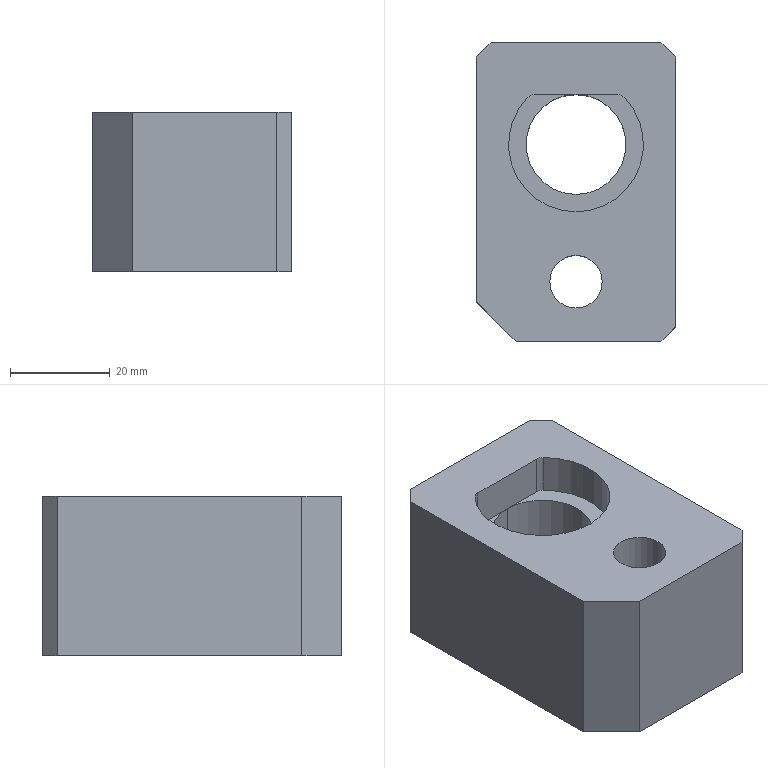Part | STEP file | lll_id3638_x_t | 1 solid | 21 faces | box 40 x 60 x 32 mm | volume 58416 mm3 | plane 13 | cylinder 8 | commonest cylinder face diameters 4 x2 20 x2 27 x2 10.5 x1 17 x1
STEP:
#1=CARTESIAN_POINT('',(3587.234,240.45,60.5));
#2=VERTEX_POINT('',#1);
#3=CARTESIAN_POINT('',(3587.234,220.45,60.5));
#4=VERTEX_POINT('',#3);
#5=CARTESIAN_POINT('',(3587.234,230.45,60.5));
#6=DIRECTION('',(0.,0.,-1.));
#7=DIRECTION('',(1.,0.,0.));
#8=AXIS2_PLACEMENT_3D('',#5,#6,#7);
#9=CIRCLE('',#8,10.);
#10=EDGE_CURVE('',#2,#4,#9,.T.);
#11=ORIENTED_EDGE('',*,*,#10,.F.);
#12=CARTESIAN_POINT('',(3587.234,230.45,60.5));
#13=DIRECTION('',(0.,0.,-1.));
#14=DIRECTION('',(1.,0.,0.));
#15=AXIS2_PLACEMENT_3D('',#12,#13,#14);
#16=CIRCLE('',#15,10.);
#17=EDGE_CURVE('',#4,#2,#16,.T.);
#18=ORIENTED_EDGE('',*,*,#17,.F.);
#19=EDGE_LOOP('',(#11,#18));
#20=FACE_BOUND('',#19,.T.);
#21=CARTESIAN_POINT('',(3567.234,198.95,60.5));
#22=VERTEX_POINT('',#21);
#23=CARTESIAN_POINT('',(3567.234,247.95,60.5));
#24=VERTEX_POINT('',#23);
#25=CARTESIAN_POINT('',(3567.234,199.225,60.5));
#26=DIRECTION('',(0.,1.,0.));
#27=VECTOR('',#26,1.);
#28=LINE('',#25,#27);
#29=EDGE_CURVE('',#22,#24,#28,.T.);
#30=ORIENTED_EDGE('',*,*,#29,.T.);
#31=CARTESIAN_POINT('',(3570.234,250.95,60.5));
#32=VERTEX_POINT('',#31);
#33=CARTESIAN_POINT('',(3570.234,250.95,60.5));
#34=DIRECTION('',(-0.7071,-0.7071,0.));
#35=VECTOR('',#34,1.);
#36=LINE('',#33,#35);
#37=EDGE_CURVE('',#32,#24,#36,.T.);
#38=ORIENTED_EDGE('',*,*,#37,.F.);
#39=CARTESIAN_POINT('',(3604.234,250.95,60.5));
#40=VERTEX_POINT('',#39);
#41=CARTESIAN_POINT('',(3587.234,250.95,60.5));
#42=DIRECTION('',(1.,0.,0.));
#43=VECTOR('',#42,1.);
#44=LINE('',#41,#43);
#45=EDGE_CURVE('',#32,#40,#44,.T.);
#46=ORIENTED_EDGE('',*,*,#45,.T.);
#47=CARTESIAN_POINT('',(3607.234,247.95,60.5));
#48=VERTEX_POINT('',#47);
#49=CARTESIAN_POINT('',(3607.234,247.95,60.5));
#50=DIRECTION('',(-0.7071,0.7071,0.));
#51=VECTOR('',#50,1.);
#52=LINE('',#49,#51);
#53=EDGE_CURVE('',#48,#40,#52,.T.);
#54=ORIENTED_EDGE('',*,*,#53,.F.);
#55=CARTESIAN_POINT('',(3607.234,193.95,60.5));
#56=VERTEX_POINT('',#55);
#57=CARTESIAN_POINT('',(3607.234,199.225,60.5));
#58=DIRECTION('',(0.,-1.,0.));
#59=VECTOR('',#58,1.);
#60=LINE('',#57,#59);
#61=EDGE_CURVE('',#48,#56,#60,.T.);
#62=ORIENTED_EDGE('',*,*,#61,.T.);
#63=CARTESIAN_POINT('',(3604.234,190.95,60.5));
#64=VERTEX_POINT('',#63);
#65=CARTESIAN_POINT('',(3604.234,190.95,60.5));
#66=DIRECTION('',(0.7071,0.7071,0.));
#67=VECTOR('',#66,1.);
#68=LINE('',#65,#67);
#69=EDGE_CURVE('',#64,#56,#68,.T.);
#70=ORIENTED_EDGE('',*,*,#69,.F.);
#71=CARTESIAN_POINT('',(3575.234,190.95,60.5));
#72=VERTEX_POINT('',#71);
#73=CARTESIAN_POINT('',(3587.234,190.95,60.5));
#74=DIRECTION('',(-1.,0.,0.));
#75=VECTOR('',#74,1.);
#76=LINE('',#73,#75);
#77=EDGE_CURVE('',#64,#72,#76,.T.);
#78=ORIENTED_EDGE('',*,*,#77,.T.);
#79=CARTESIAN_POINT('',(3575.234,190.95,60.5));
#80=DIRECTION('',(0.7071,-0.7071,0.));
#81=VECTOR('',#80,1.);
#82=LINE('',#79,#81);
#83=EDGE_CURVE('',#22,#72,#82,.T.);
#84=ORIENTED_EDGE('',*,*,#83,.F.);
#85=EDGE_LOOP('',(#30,#38,#46,#54,#62,#70,#78,#84));
#86=FACE_BOUND('',#85,.T.);
#87=CARTESIAN_POINT('',(3595.734,202.95,60.5));
#88=VERTEX_POINT('',#87);
#89=CARTESIAN_POINT('',(3587.234,202.95,60.5));
#90=DIRECTION('',(0.,0.,-1.));
#91=DIRECTION('',(1.,0.,0.));
#92=AXIS2_PLACEMENT_3D('',#89,#90,#91);
#93=CIRCLE('',#92,8.5);
#94=EDGE_CURVE('',#88,#88,#93,.T.);
#95=ORIENTED_EDGE('',*,*,#94,.F.);
#96=EDGE_LOOP('',(#95));
#97=FACE_BOUND('',#96,.T.);
#98=CARTESIAN_POINT('',(3655.374,199.225,60.5));
#99=DIRECTION('',(0.,0.,1.));
#100=DIRECTION('',(1.,0.,0.));
#101=AXIS2_PLACEMENT_3D('',#98,#99,#100);
#102=PLANE('',#101);
#103=ADVANCED_FACE('',(#20,#86,#97),#102,.F.);
#104=CARTESIAN_POINT('',(3595.495,240.45,92.5));
#105=VERTEX_POINT('',#104);
#106=CARTESIAN_POINT('',(3578.973,240.45,92.5));
#107=VERTEX_POINT('',#106);
#108=CARTESIAN_POINT('',(3581.484,240.45,92.5));
#109=DIRECTION('',(-1.,0.,0.));
#110=VECTOR('',#109,1.);
#111=LINE('',#108,#110);
#112=EDGE_CURVE('',#105,#107,#111,.T.);
#113=ORIENTED_EDGE('',*,*,#112,.F.);
#114=CARTESIAN_POINT('',(3596.932,239.841,92.5));
#115=VERTEX_POINT('',#114);
#116=CARTESIAN_POINT('',(3595.495,238.45,92.5));
#117=DIRECTION('',(0.,0.,-1.));
#118=DIRECTION('',(1.,0.,0.));
#119=AXIS2_PLACEMENT_3D('',#116,#117,#118);
#120=CIRCLE('',#119,2.);
#121=EDGE_CURVE('',#105,#115,#120,.T.);
#122=ORIENTED_EDGE('',*,*,#121,.T.);
#123=CARTESIAN_POINT('',(3587.234,216.95,92.5));
#124=VERTEX_POINT('',#123);
#125=CARTESIAN_POINT('',(3587.234,230.45,92.5));
#126=DIRECTION('',(0.,0.,1.));
#127=DIRECTION('',(1.,0.,0.));
#128=AXIS2_PLACEMENT_3D('',#125,#126,#127);
#129=CIRCLE('',#128,13.5);
#130=EDGE_CURVE('',#124,#115,#129,.T.);
#131=ORIENTED_EDGE('',*,*,#130,.F.);
#132=CARTESIAN_POINT('',(3577.536,239.841,92.5));
#133=VERTEX_POINT('',#132);
#134=CARTESIAN_POINT('',(3587.234,230.45,92.5));
#135=DIRECTION('',(0.,0.,1.));
#136=DIRECTION('',(1.,0.,0.));
#137=AXIS2_PLACEMENT_3D('',#134,#135,#136);
#138=CIRCLE('',#137,13.5);
#139=EDGE_CURVE('',#133,#124,#138,.T.);
#140=ORIENTED_EDGE('',*,*,#139,.F.);
#141=CARTESIAN_POINT('',(3578.973,238.45,92.5));
#142=DIRECTION('',(0.,0.,-1.));
#143=DIRECTION('',(1.,0.,0.));
#144=AXIS2_PLACEMENT_3D('',#141,#142,#143);
#145=CIRCLE('',#144,2.);
#146=EDGE_CURVE('',#133,#107,#145,.T.);
#147=ORIENTED_EDGE('',*,*,#146,.T.);
#148=EDGE_LOOP('',(#113,#122,#131,#140,#147));
#149=FACE_BOUND('',#148,.T.);
#150=CARTESIAN_POINT('',(3592.484,202.95,92.5));
#151=VERTEX_POINT('',#150);
#152=CARTESIAN_POINT('',(3587.234,202.95,92.5));
#153=DIRECTION('',(0.,0.,-1.));
#154=DIRECTION('',(1.,0.,0.));
#155=AXIS2_PLACEMENT_3D('',#152,#153,#154);
#156=CIRCLE('',#155,5.25);
#157=EDGE_CURVE('',#151,#151,#156,.T.);
#158=ORIENTED_EDGE('',*,*,#157,.T.);
#159=EDGE_LOOP('',(#158));
#160=FACE_BOUND('',#159,.T.);
#161=CARTESIAN_POINT('',(3575.234,190.95,92.5));
#162=VERTEX_POINT('',#161);
#163=CARTESIAN_POINT('',(3604.234,190.95,92.5));
#164=VERTEX_POINT('',#163);
#165=CARTESIAN_POINT('',(3587.234,190.95,92.5));
#166=DIRECTION('',(1.,0.,0.));
#167=VECTOR('',#166,1.);
#168=LINE('',#165,#167);
#169=EDGE_CURVE('',#162,#164,#168,.T.);
#170=ORIENTED_EDGE('',*,*,#169,.T.);
#171=CARTESIAN_POINT('',(3607.234,193.95,92.5));
#172=VERTEX_POINT('',#171);
#173=CARTESIAN_POINT('',(3604.234,190.95,92.5));
#174=DIRECTION('',(-0.7071,-0.7071,0.));
#175=VECTOR('',#174,1.);
#176=LINE('',#173,#175);
#177=EDGE_CURVE('',#172,#164,#176,.T.);
#178=ORIENTED_EDGE('',*,*,#177,.F.);
#179=CARTESIAN_POINT('',(3607.234,247.95,92.5));
#180=VERTEX_POINT('',#179);
#181=CARTESIAN_POINT('',(3607.234,199.225,92.5));
#182=DIRECTION('',(0.,1.,0.));
#183=VECTOR('',#182,1.);
#184=LINE('',#181,#183);
#185=EDGE_CURVE('',#172,#180,#184,.T.);
#186=ORIENTED_EDGE('',*,*,#185,.T.);
#187=CARTESIAN_POINT('',(3604.234,250.95,92.5));
#188=VERTEX_POINT('',#187);
#189=CARTESIAN_POINT('',(3607.234,247.95,92.5));
#190=DIRECTION('',(0.7071,-0.7071,0.));
#191=VECTOR('',#190,1.);
#192=LINE('',#189,#191);
#193=EDGE_CURVE('',#188,#180,#192,.T.);
#194=ORIENTED_EDGE('',*,*,#193,.F.);
#195=CARTESIAN_POINT('',(3570.234,250.95,92.5));
#196=VERTEX_POINT('',#195);
#197=CARTESIAN_POINT('',(3587.234,250.95,92.5));
#198=DIRECTION('',(-1.,0.,0.));
#199=VECTOR('',#198,1.);
#200=LINE('',#197,#199);
#201=EDGE_CURVE('',#188,#196,#200,.T.);
#202=ORIENTED_EDGE('',*,*,#201,.T.);
#203=CARTESIAN_POINT('',(3567.234,247.95,92.5));
#204=VERTEX_POINT('',#203);
#205=CARTESIAN_POINT('',(3570.234,250.95,92.5));
#206=DIRECTION('',(0.7071,0.7071,0.));
#207=VECTOR('',#206,1.);
#208=LINE('',#205,#207);
#209=EDGE_CURVE('',#204,#196,#208,.T.);
#210=ORIENTED_EDGE('',*,*,#209,.F.);
#211=CARTESIAN_POINT('',(3567.234,198.95,92.5));
#212=VERTEX_POINT('',#211);
#213=CARTESIAN_POINT('',(3567.234,199.225,92.5));
#214=DIRECTION('',(0.,-1.,0.));
#215=VECTOR('',#214,1.);
#216=LINE('',#213,#215);
#217=EDGE_CURVE('',#204,#212,#216,.T.);
#218=ORIENTED_EDGE('',*,*,#217,.T.);
#219=CARTESIAN_POINT('',(3575.234,190.95,92.5));
#220=DIRECTION('',(-0.7071,0.7071,0.));
#221=VECTOR('',#220,1.);
#222=LINE('',#219,#221);
#223=EDGE_CURVE('',#162,#212,#222,.T.);
#224=ORIENTED_EDGE('',*,*,#223,.F.);
#225=EDGE_LOOP('',(#170,#178,#186,#194,#202,#210,#218,#224));
#226=FACE_BOUND('',#225,.T.);
#227=CARTESIAN_POINT('',(3655.374,199.225,92.5));
#228=DIRECTION('',(0.,0.,1.));
#229=DIRECTION('',(1.,0.,0.));
#230=AXIS2_PLACEMENT_3D('',#227,#228,#229);
#231=PLANE('',#230);
#232=ADVANCED_FACE('',(#149,#160,#226),#231,.T.);
#233=ORIENTED_EDGE('',*,*,#201,.F.);
#234=CARTESIAN_POINT('',(3604.234,250.95,-8.5));
#235=DIRECTION('',(0.,0.,1.));
#236=VECTOR('',#235,1.);
#237=LINE('',#234,#236);
#238=EDGE_CURVE('',#40,#188,#237,.T.);
#239=ORIENTED_EDGE('',*,*,#238,.F.);
#240=ORIENTED_EDGE('',*,*,#45,.F.);
#241=CARTESIAN_POINT('',(3570.234,250.95,-8.5));
#242=DIRECTION('',(0.,0.,-1.));
#243=VECTOR('',#242,1.);
#244=LINE('',#241,#243);
#245=EDGE_CURVE('',#196,#32,#244,.T.);
#246=ORIENTED_EDGE('',*,*,#245,.F.);
#247=EDGE_LOOP('',(#233,#239,#240,#246));
#248=FACE_OUTER_BOUND('',#247,.T.);
#249=CARTESIAN_POINT('',(3587.234,250.95,-8.5));
#250=DIRECTION('',(0.,1.,0.));
#251=DIRECTION('',(0.,0.,-1.));
#252=AXIS2_PLACEMENT_3D('',#249,#250,#251);
#253=PLANE('',#252);
#254=ADVANCED_FACE('',(#248),#253,.T.);
#255=ORIENTED_EDGE('',*,*,#217,.F.);
#256=CARTESIAN_POINT('',(3567.234,247.95,-8.5));
#257=DIRECTION('',(0.,0.,1.));
#258=VECTOR('',#257,1.);
#259=LINE('',#256,#258);
#260=EDGE_CURVE('',#24,#204,#259,.T.);
#261=ORIENTED_EDGE('',*,*,#260,.F.);
#262=ORIENTED_EDGE('',*,*,#29,.F.);
#263=CARTESIAN_POINT('',(3567.234,198.95,-8.5));
#264=DIRECTION('',(0.,0.,-1.));
#265=VECTOR('',#264,1.);
#266=LINE('',#263,#265);
#267=EDGE_CURVE('',#212,#22,#266,.T.);
#268=ORIENTED_EDGE('',*,*,#267,.F.);
#269=EDGE_LOOP('',(#255,#261,#262,#268));
#270=FACE_OUTER_BOUND('',#269,.T.);
#271=CARTESIAN_POINT('',(3567.234,230.45,-8.5));
#272=DIRECTION('',(-1.,0.,0.));
#273=DIRECTION('',(0.,0.,1.));
#274=AXIS2_PLACEMENT_3D('',#271,#272,#273);
#275=PLANE('',#274);
#276=ADVANCED_FACE('',(#270),#275,.T.);
#277=ORIENTED_EDGE('',*,*,#77,.F.);
#278=CARTESIAN_POINT('',(3604.234,190.95,-8.5));
#279=DIRECTION('',(0.,0.,-1.));
#280=VECTOR('',#279,1.);
#281=LINE('',#278,#280);
#282=EDGE_CURVE('',#164,#64,#281,.T.);
#283=ORIENTED_EDGE('',*,*,#282,.F.);
#284=ORIENTED_EDGE('',*,*,#169,.F.);
#285=CARTESIAN_POINT('',(3575.234,190.95,-8.5));
#286=DIRECTION('',(0.,0.,1.));
#287=VECTOR('',#286,1.);
#288=LINE('',#285,#287);
#289=EDGE_CURVE('',#72,#162,#288,.T.);
#290=ORIENTED_EDGE('',*,*,#289,.F.);
#291=EDGE_LOOP('',(#277,#283,#284,#290));
#292=FACE_OUTER_BOUND('',#291,.T.);
#293=CARTESIAN_POINT('',(3587.234,190.95,-8.5));
#294=DIRECTION('',(0.,-1.,0.));
#295=DIRECTION('',(0.,0.,1.));
#296=AXIS2_PLACEMENT_3D('',#293,#294,#295);
#297=PLANE('',#296);
#298=ADVANCED_FACE('',(#292),#297,.T.);
#299=ORIENTED_EDGE('',*,*,#61,.F.);
#300=CARTESIAN_POINT('',(3607.234,247.95,-8.5));
#301=DIRECTION('',(0.,0.,-1.));
#302=VECTOR('',#301,1.);
#303=LINE('',#300,#302);
#304=EDGE_CURVE('',#180,#48,#303,.T.);
#305=ORIENTED_EDGE('',*,*,#304,.F.);
#306=ORIENTED_EDGE('',*,*,#185,.F.);
#307=CARTESIAN_POINT('',(3607.234,193.95,-8.5));
#308=DIRECTION('',(0.,0.,1.));
#309=VECTOR('',#308,1.);
#310=LINE('',#307,#309);
#311=EDGE_CURVE('',#56,#172,#310,.T.);
#312=ORIENTED_EDGE('',*,*,#311,.F.);
#313=EDGE_LOOP('',(#299,#305,#306,#312));
#314=FACE_OUTER_BOUND('',#313,.T.);
#315=CARTESIAN_POINT('',(3607.234,230.45,-8.5));
#316=DIRECTION('',(1.,0.,0.));
#317=DIRECTION('',(0.,0.,-1.));
#318=AXIS2_PLACEMENT_3D('',#315,#316,#317);
#319=PLANE('',#318);
#320=ADVANCED_FACE('',(#314),#319,.T.);
#321=ORIENTED_EDGE('',*,*,#157,.F.);
#322=EDGE_LOOP('',(#321));
#323=FACE_BOUND('',#322,.T.);
#324=CARTESIAN_POINT('',(3592.484,202.95,77.5));
#325=VERTEX_POINT('',#324);
#326=CARTESIAN_POINT('',(3587.234,202.95,77.5));
#327=DIRECTION('',(0.,0.,1.));
#328=DIRECTION('',(1.,0.,0.));
#329=AXIS2_PLACEMENT_3D('',#326,#327,#328);
#330=CIRCLE('',#329,5.25);
#331=EDGE_CURVE('',#325,#325,#330,.T.);
#332=ORIENTED_EDGE('',*,*,#331,.F.);
#333=EDGE_LOOP('',(#332));
#334=FACE_BOUND('',#333,.T.);
#335=CARTESIAN_POINT('',(3587.234,202.95,160.5));
#336=DIRECTION('',(0.,0.,1.));
#337=DIRECTION('',(1.,0.,0.));
#338=AXIS2_PLACEMENT_3D('',#335,#336,#337);
#339=CYLINDRICAL_SURFACE('',#338,5.25);
#340=ADVANCED_FACE('',(#323,#334),#339,.F.);
#341=ORIENTED_EDGE('',*,*,#331,.T.);
#342=EDGE_LOOP('',(#341));
#343=FACE_BOUND('',#342,.T.);
#344=CARTESIAN_POINT('',(3595.734,202.95,77.5));
#345=VERTEX_POINT('',#344);
#346=CARTESIAN_POINT('',(3587.234,202.95,77.5));
#347=DIRECTION('',(0.,0.,1.));
#348=DIRECTION('',(1.,0.,0.));
#349=AXIS2_PLACEMENT_3D('',#346,#347,#348);
#350=CIRCLE('',#349,8.5);
#351=EDGE_CURVE('',#345,#345,#350,.T.);
#352=ORIENTED_EDGE('',*,*,#351,.F.);
#353=EDGE_LOOP('',(#352));
#354=FACE_BOUND('',#353,.T.);
#355=CARTESIAN_POINT('',(3587.234,202.95,77.5));
#356=DIRECTION('',(0.,0.,1.));
#357=DIRECTION('',(1.,0.,0.));
#358=AXIS2_PLACEMENT_3D('',#355,#356,#357);
#359=PLANE('',#358);
#360=ADVANCED_FACE('',(#343,#354),#359,.F.);
#361=ORIENTED_EDGE('',*,*,#351,.T.);
#362=EDGE_LOOP('',(#361));
#363=FACE_BOUND('',#362,.T.);
#364=ORIENTED_EDGE('',*,*,#94,.T.);
#365=EDGE_LOOP('',(#364));
#366=FACE_BOUND('',#365,.T.);
#367=CARTESIAN_POINT('',(3587.234,202.95,60.5));
#368=DIRECTION('',(0.,0.,1.));
#369=DIRECTION('',(1.,0.,0.));
#370=AXIS2_PLACEMENT_3D('',#367,#368,#369);
#371=CYLINDRICAL_SURFACE('',#370,8.5);
#372=ADVANCED_FACE('',(#363,#366),#371,.F.);
#373=ORIENTED_EDGE('',*,*,#177,.T.);
#374=ORIENTED_EDGE('',*,*,#282,.T.);
#375=ORIENTED_EDGE('',*,*,#69,.T.);
#376=ORIENTED_EDGE('',*,*,#311,.T.);
#377=EDGE_LOOP('',(#373,#374,#375,#376));
#378=FACE_OUTER_BOUND('',#377,.T.);
#379=CARTESIAN_POINT('',(3604.234,190.95,-8.5));
#380=DIRECTION('',(-0.7071,0.7071,0.));
#381=DIRECTION('',(-0.7071,-0.7071,0.));
#382=AXIS2_PLACEMENT_3D('',#379,#380,#381);
#383=PLANE('',#382);
#384=ADVANCED_FACE('',(#378),#383,.F.);
#385=ORIENTED_EDGE('',*,*,#209,.T.);
#386=ORIENTED_EDGE('',*,*,#245,.T.);
#387=ORIENTED_EDGE('',*,*,#37,.T.);
#388=ORIENTED_EDGE('',*,*,#260,.T.);
#389=EDGE_LOOP('',(#385,#386,#387,#388));
#390=FACE_OUTER_BOUND('',#389,.T.);
#391=CARTESIAN_POINT('',(3570.234,250.95,-8.5));
#392=DIRECTION('',(0.7071,-0.7071,0.));
#393=DIRECTION('',(0.7071,0.7071,0.));
#394=AXIS2_PLACEMENT_3D('',#391,#392,#393);
#395=PLANE('',#394);
#396=ADVANCED_FACE('',(#390),#395,.F.);
#397=ORIENTED_EDGE('',*,*,#193,.T.);
#398=ORIENTED_EDGE('',*,*,#304,.T.);
#399=ORIENTED_EDGE('',*,*,#53,.T.);
#400=ORIENTED_EDGE('',*,*,#238,.T.);
#401=EDGE_LOOP('',(#397,#398,#399,#400));
#402=FACE_OUTER_BOUND('',#401,.T.);
#403=CARTESIAN_POINT('',(3607.234,247.95,-8.5));
#404=DIRECTION('',(-0.7071,-0.7071,0.));
#405=DIRECTION('',(0.7071,-0.7071,0.));
#406=AXIS2_PLACEMENT_3D('',#403,#404,#405);
#407=PLANE('',#406);
#408=ADVANCED_FACE('',(#402),#407,.F.);
#409=ORIENTED_EDGE('',*,*,#83,.T.);
#410=ORIENTED_EDGE('',*,*,#289,.T.);
#411=ORIENTED_EDGE('',*,*,#223,.T.);
#412=ORIENTED_EDGE('',*,*,#267,.T.);
#413=EDGE_LOOP('',(#409,#410,#411,#412));
#414=FACE_OUTER_BOUND('',#413,.T.);
#415=CARTESIAN_POINT('',(3575.234,190.95,-8.5));
#416=DIRECTION('',(0.7071,0.7071,0.));
#417=DIRECTION('',(-0.7071,0.7071,0.));
#418=AXIS2_PLACEMENT_3D('',#415,#416,#417);
#419=PLANE('',#418);
#420=ADVANCED_FACE('',(#414),#419,.F.);
#421=ORIENTED_EDGE('',*,*,#10,.T.);
#422=CARTESIAN_POINT('',(3587.234,220.45,84.5));
#423=VERTEX_POINT('',#422);
#424=CARTESIAN_POINT('',(3587.234,220.45,38.5));
#425=DIRECTION('',(0.,0.,-1.));
#426=VECTOR('',#425,1.);
#427=LINE('',#424,#426);
#428=EDGE_CURVE('',#423,#4,#427,.T.);
#429=ORIENTED_EDGE('',*,*,#428,.F.);
#430=CARTESIAN_POINT('',(3587.234,240.45,84.5));
#431=VERTEX_POINT('',#430);
#432=CARTESIAN_POINT('',(3587.234,230.45,84.5));
#433=DIRECTION('',(0.,0.,-1.));
#434=DIRECTION('',(0.,-1.,0.));
#435=AXIS2_PLACEMENT_3D('',#432,#433,#434);
#436=CIRCLE('',#435,10.);
#437=EDGE_CURVE('',#431,#423,#436,.T.);
#438=ORIENTED_EDGE('',*,*,#437,.F.);
#439=CARTESIAN_POINT('',(3587.234,240.45,38.5));
#440=DIRECTION('',(0.,0.,1.));
#441=VECTOR('',#440,1.);
#442=LINE('',#439,#441);
#443=EDGE_CURVE('',#2,#431,#442,.T.);
#444=ORIENTED_EDGE('',*,*,#443,.F.);
#445=EDGE_LOOP('',(#421,#429,#438,#444));
#446=FACE_OUTER_BOUND('',#445,.T.);
#447=CARTESIAN_POINT('',(3587.234,230.45,38.5));
#448=DIRECTION('',(0.,0.,-1.));
#449=DIRECTION('',(0.,1.,0.));
#450=AXIS2_PLACEMENT_3D('',#447,#448,#449);
#451=CYLINDRICAL_SURFACE('',#450,10.);
#452=ADVANCED_FACE('',(#446),#451,.F.);
#453=ORIENTED_EDGE('',*,*,#130,.T.);
#454=CARTESIAN_POINT('',(3596.932,239.841,84.5));
#455=VERTEX_POINT('',#454);
#456=CARTESIAN_POINT('',(3596.932,239.841,88.5));
#457=DIRECTION('',(0.,0.,-1.));
#458=VECTOR('',#457,1.);
#459=LINE('',#456,#458);
#460=EDGE_CURVE('',#115,#455,#459,.T.);
#461=ORIENTED_EDGE('',*,*,#460,.T.);
#462=CARTESIAN_POINT('',(3587.234,216.95,84.5));
#463=VERTEX_POINT('',#462);
#464=CARTESIAN_POINT('',(3587.234,230.45,84.5));
#465=DIRECTION('',(0.,0.,-1.));
#466=DIRECTION('',(-1.,0.,0.));
#467=AXIS2_PLACEMENT_3D('',#464,#465,#466);
#468=CIRCLE('',#467,13.5);
#469=EDGE_CURVE('',#455,#463,#468,.T.);
#470=ORIENTED_EDGE('',*,*,#469,.T.);
#471=CARTESIAN_POINT('',(3587.234,216.95,88.5));
#472=DIRECTION('',(0.,0.,-1.));
#473=VECTOR('',#472,1.);
#474=LINE('',#471,#473);
#475=EDGE_CURVE('',#124,#463,#474,.T.);
#476=ORIENTED_EDGE('',*,*,#475,.F.);
#477=EDGE_LOOP('',(#453,#461,#470,#476));
#478=FACE_OUTER_BOUND('',#477,.T.);
#479=CARTESIAN_POINT('',(3587.234,230.45,88.5));
#480=DIRECTION('',(0.,0.,-1.));
#481=DIRECTION('',(0.,1.,0.));
#482=AXIS2_PLACEMENT_3D('',#479,#480,#481);
#483=CYLINDRICAL_SURFACE('',#482,13.5);
#484=ADVANCED_FACE('',(#478),#483,.F.);
#485=CARTESIAN_POINT('',(3595.495,240.45,84.5));
#486=VERTEX_POINT('',#485);
#487=CARTESIAN_POINT('',(3581.484,240.45,84.5));
#488=DIRECTION('',(-1.,0.,0.));
#489=VECTOR('',#488,1.);
#490=LINE('',#487,#489);
#491=EDGE_CURVE('',#486,#431,#490,.T.);
#492=ORIENTED_EDGE('',*,*,#491,.F.);
#493=CARTESIAN_POINT('',(3595.495,240.45,92.51));
#494=DIRECTION('',(0.,0.,1.));
#495=VECTOR('',#494,1.);
#496=LINE('',#493,#495);
#497=EDGE_CURVE('',#486,#105,#496,.T.);
#498=ORIENTED_EDGE('',*,*,#497,.T.);
#499=ORIENTED_EDGE('',*,*,#112,.T.);
#500=CARTESIAN_POINT('',(3578.973,240.45,84.5));
#501=VERTEX_POINT('',#500);
#502=CARTESIAN_POINT('',(3578.973,240.45,92.51));
#503=DIRECTION('',(0.,0.,-1.));
#504=VECTOR('',#503,1.);
#505=LINE('',#502,#504);
#506=EDGE_CURVE('',#107,#501,#505,.T.);
#507=ORIENTED_EDGE('',*,*,#506,.T.);
#508=CARTESIAN_POINT('',(3581.484,240.45,84.5));
#509=DIRECTION('',(-1.,0.,0.));
#510=VECTOR('',#509,1.);
#511=LINE('',#508,#510);
#512=EDGE_CURVE('',#431,#501,#511,.T.);
#513=ORIENTED_EDGE('',*,*,#512,.F.);
#514=EDGE_LOOP('',(#492,#498,#499,#507,#513));
#515=FACE_OUTER_BOUND('',#514,.T.);
#516=CARTESIAN_POINT('',(3575.734,240.45,92.51));
#517=DIRECTION('',(0.,-1.,0.));
#518=DIRECTION('',(1.,0.,0.));
#519=AXIS2_PLACEMENT_3D('',#516,#517,#518);
#520=PLANE('',#519);
#521=ADVANCED_FACE('',(#515),#520,.T.);
#522=CARTESIAN_POINT('',(3577.536,239.841,84.5));
#523=VERTEX_POINT('',#522);
#524=CARTESIAN_POINT('',(3587.234,230.45,84.5));
#525=DIRECTION('',(0.,0.,-1.));
#526=DIRECTION('',(-1.,0.,0.));
#527=AXIS2_PLACEMENT_3D('',#524,#525,#526);
#528=CIRCLE('',#527,13.5);
#529=EDGE_CURVE('',#463,#523,#528,.T.);
#530=ORIENTED_EDGE('',*,*,#529,.T.);
#531=CARTESIAN_POINT('',(3577.536,239.841,88.5));
#532=DIRECTION('',(0.,0.,1.));
#533=VECTOR('',#532,1.);
#534=LINE('',#531,#533);
#535=EDGE_CURVE('',#523,#133,#534,.T.);
#536=ORIENTED_EDGE('',*,*,#535,.T.);
#537=ORIENTED_EDGE('',*,*,#139,.T.);
#538=ORIENTED_EDGE('',*,*,#475,.T.);
#539=EDGE_LOOP('',(#530,#536,#537,#538));
#540=FACE_OUTER_BOUND('',#539,.T.);
#541=CARTESIAN_POINT('',(3587.234,230.45,88.5));
#542=DIRECTION('',(0.,0.,-1.));
#543=DIRECTION('',(0.,1.,0.));
#544=AXIS2_PLACEMENT_3D('',#541,#542,#543);
#545=CYLINDRICAL_SURFACE('',#544,13.5);
#546=ADVANCED_FACE('',(#540),#545,.F.);
#547=ORIENTED_EDGE('',*,*,#469,.F.);
#548=CARTESIAN_POINT('',(3595.495,238.45,84.5));
#549=DIRECTION('',(0.,0.,1.));
#550=DIRECTION('',(-1.,0.,0.));
#551=AXIS2_PLACEMENT_3D('',#548,#549,#550);
#552=CIRCLE('',#551,2.);
#553=EDGE_CURVE('',#455,#486,#552,.T.);
#554=ORIENTED_EDGE('',*,*,#553,.T.);
#555=ORIENTED_EDGE('',*,*,#491,.T.);
#556=ORIENTED_EDGE('',*,*,#437,.T.);
#557=CARTESIAN_POINT('',(3587.234,230.45,84.5));
#558=DIRECTION('',(0.,0.,-1.));
#559=DIRECTION('',(0.,-1.,0.));
#560=AXIS2_PLACEMENT_3D('',#557,#558,#559);
#561=CIRCLE('',#560,10.);
#562=EDGE_CURVE('',#423,#431,#561,.T.);
#563=ORIENTED_EDGE('',*,*,#562,.T.);
#564=ORIENTED_EDGE('',*,*,#512,.T.);
#565=CARTESIAN_POINT('',(3578.973,238.45,84.5));
#566=DIRECTION('',(0.,0.,1.));
#567=DIRECTION('',(-1.,0.,0.));
#568=AXIS2_PLACEMENT_3D('',#565,#566,#567);
#569=CIRCLE('',#568,2.);
#570=EDGE_CURVE('',#501,#523,#569,.T.);
#571=ORIENTED_EDGE('',*,*,#570,.T.);
#572=ORIENTED_EDGE('',*,*,#529,.F.);
#573=EDGE_LOOP('',(#547,#554,#555,#556,#563,#564,#571,#572));
#574=FACE_OUTER_BOUND('',#573,.T.);
#575=CARTESIAN_POINT('',(3587.234,219.2,84.5));
#576=DIRECTION('',(0.,0.,-1.));
#577=DIRECTION('',(0.,-1.,0.));
#578=AXIS2_PLACEMENT_3D('',#575,#576,#577);
#579=PLANE('',#578);
#580=ADVANCED_FACE('',(#574),#579,.F.);
#581=ORIENTED_EDGE('',*,*,#17,.T.);
#582=ORIENTED_EDGE('',*,*,#443,.T.);
#583=ORIENTED_EDGE('',*,*,#562,.F.);
#584=ORIENTED_EDGE('',*,*,#428,.T.);
#585=EDGE_LOOP('',(#581,#582,#583,#584));
#586=FACE_OUTER_BOUND('',#585,.T.);
#587=CARTESIAN_POINT('',(3587.234,230.45,38.5));
#588=DIRECTION('',(0.,0.,-1.));
#589=DIRECTION('',(0.,1.,0.));
#590=AXIS2_PLACEMENT_3D('',#587,#588,#589);
#591=CYLINDRICAL_SURFACE('',#590,10.);
#592=ADVANCED_FACE('',(#586),#591,.F.);
#593=ORIENTED_EDGE('',*,*,#121,.F.);
#594=ORIENTED_EDGE('',*,*,#497,.F.);
#595=ORIENTED_EDGE('',*,*,#553,.F.);
#596=ORIENTED_EDGE('',*,*,#460,.F.);
#597=EDGE_LOOP('',(#593,#594,#595,#596));
#598=FACE_OUTER_BOUND('',#597,.T.);
#599=CARTESIAN_POINT('',(3595.495,238.45,88.5));
#600=DIRECTION('',(0.,0.,-1.));
#601=DIRECTION('',(-1.,0.,0.));
#602=AXIS2_PLACEMENT_3D('',#599,#600,#601);
#603=CYLINDRICAL_SURFACE('',#602,2.);
#604=ADVANCED_FACE('',(#598),#603,.F.);
#605=ORIENTED_EDGE('',*,*,#570,.F.);
#606=ORIENTED_EDGE('',*,*,#506,.F.);
#607=ORIENTED_EDGE('',*,*,#146,.F.);
#608=ORIENTED_EDGE('',*,*,#535,.F.);
#609=EDGE_LOOP('',(#605,#606,#607,#608));
#610=FACE_OUTER_BOUND('',#609,.T.);
#611=CARTESIAN_POINT('',(3578.973,238.45,88.5));
#612=DIRECTION('',(0.,0.,-1.));
#613=DIRECTION('',(-1.,0.,0.));
#614=AXIS2_PLACEMENT_3D('',#611,#612,#613);
#615=CYLINDRICAL_SURFACE('',#614,2.);
#616=ADVANCED_FACE('',(#610),#615,.F.);
#617=CLOSED_SHELL('',(#103,#232,#254,#276,#298,#320,#340,#360,#372,#384,#396,#408,#420,#452,#484,#521,#546,#580,#592,#604,#616));
#618=MANIFOLD_SOLID_BREP('',#617);
#619=(LENGTH_UNIT()NAMED_UNIT(*)SI_UNIT(.MILLI.,.METRE.));
#620=UNCERTAINTY_MEASURE_WITH_UNIT(LENGTH_MEASURE(0.00002),#619,'','');
#621=(NAMED_UNIT(*)PLANE_ANGLE_UNIT()SI_UNIT($,.RADIAN.));
#622=PLANE_ANGLE_MEASURE_WITH_UNIT(PLANE_ANGLE_MEASURE(0.01745),#621);
#623=DIMENSIONAL_EXPONENTS(0.,0.,0.,0.,0.,0.,0.);
#624=(CONVERSION_BASED_UNIT('DEGREE',#622)NAMED_UNIT(#623)PLANE_ANGLE_UNIT());
#625=(NAMED_UNIT(*)SI_UNIT($,.STERADIAN.)SOLID_ANGLE_UNIT());
#626=(GEOMETRIC_REPRESENTATION_CONTEXT(3)GLOBAL_UNCERTAINTY_ASSIGNED_CONTEXT((#620))GLOBAL_UNIT_ASSIGNED_CONTEXT((#619,#624,#625))REPRESENTATION_CONTEXT('',''));
#627=ADVANCED_BREP_SHAPE_REPRESENTATION('',(#618),#626);